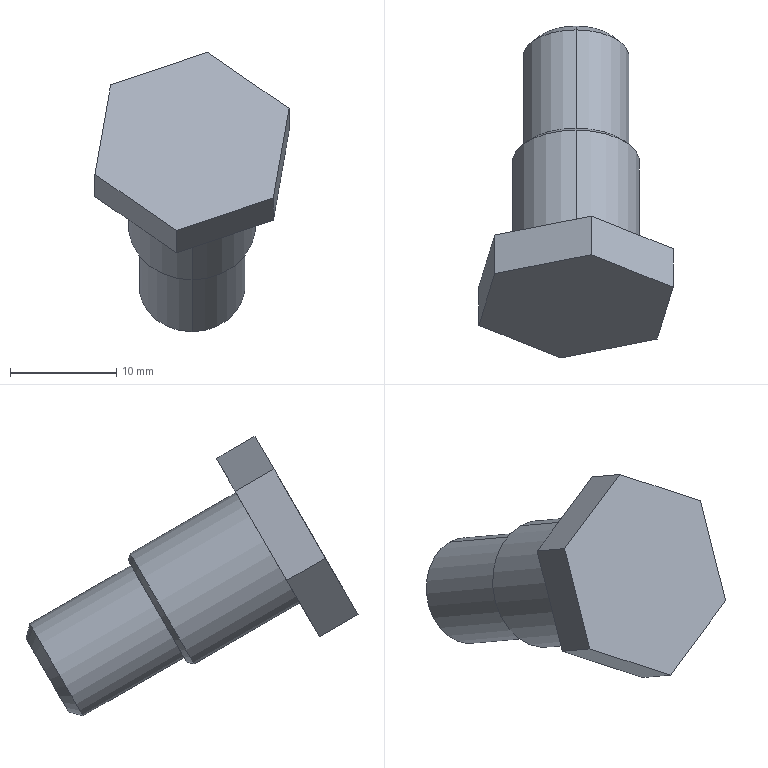Part | SolidWorks | features BaseBody 1 | 1 solid | 18 faces | box 18.291 x 31.273 x 26.332 mm | volume 3332 mm3 | plane 10 | cylinder 4 | cone 4 | commonest cylinder face diameters 10 x2 12 x2
STEP:
#1=CARTESIAN_POINT('',(-205.,-189.911,49.391));
#2=VERTEX_POINT('',#1);
#3=CARTESIAN_POINT('',(-205.,-183.911,59.783));
#4=VERTEX_POINT('',#3);
#5=CARTESIAN_POINT('',(-205.,-186.911,54.587));
#6=DIRECTION('',(0.,-0.866,0.5));
#7=DIRECTION('',(0.,-0.5,-0.866));
#8=AXIS2_PLACEMENT_3D('',#5,#6,#7);
#9=CIRCLE('',#8,6.);
#10=EDGE_CURVE('',#2,#4,#9,.T.);
#11=ORIENTED_EDGE('',*,*,#10,.T.);
#12=CARTESIAN_POINT('',(-205.,-193.871,65.533));
#13=VERTEX_POINT('',#12);
#14=CARTESIAN_POINT('',(-205.,-173.086,53.533));
#15=DIRECTION('',(0.,-0.866,0.5));
#16=VECTOR('',#15,1000.);
#17=LINE('',#14,#16);
#18=EDGE_CURVE('',#4,#13,#17,.T.);
#19=ORIENTED_EDGE('',*,*,#18,.T.);
#20=CARTESIAN_POINT('',(-205.,-199.871,55.141));
#21=VERTEX_POINT('',#20);
#22=CARTESIAN_POINT('',(-205.,-196.871,60.337));
#23=DIRECTION('',(0.,0.866,-0.5));
#24=DIRECTION('',(0.,-0.5,-0.866));
#25=AXIS2_PLACEMENT_3D('',#22,#23,#24);
#26=CIRCLE('',#25,6.);
#27=EDGE_CURVE('',#13,#21,#26,.T.);
#28=ORIENTED_EDGE('',*,*,#27,.T.);
#29=CARTESIAN_POINT('',(-205.,-179.086,43.141));
#30=DIRECTION('',(0.,-0.866,0.5));
#31=VECTOR('',#30,1000.);
#32=LINE('',#29,#31);
#33=EDGE_CURVE('',#2,#21,#32,.T.);
#34=ORIENTED_EDGE('',*,*,#33,.F.);
#35=EDGE_LOOP('',(#11,#19,#28,#34));
#36=FACE_OUTER_BOUND('',#35,.T.);
#37=CARTESIAN_POINT('',(-205.,-176.086,48.337));
#38=DIRECTION('',(0.,-0.866,0.5));
#39=DIRECTION('',(0.,-0.5,-0.866));
#40=AXIS2_PLACEMENT_3D('',#37,#38,#39);
#41=CYLINDRICAL_SURFACE('',#40,6.);
#42=ADVANCED_FACE('',(#36),#41,.T.);
#43=CARTESIAN_POINT('',(-205.,-189.228,49.574));
#44=VERTEX_POINT('',#43);
#45=CARTESIAN_POINT('',(-205.,-183.728,59.1));
#46=VERTEX_POINT('',#45);
#47=CARTESIAN_POINT('',(-205.,-186.478,54.337));
#48=DIRECTION('',(0.,-0.866,0.5));
#49=DIRECTION('',(0.,-0.5,-0.866));
#50=AXIS2_PLACEMENT_3D('',#47,#48,#49);
#51=CIRCLE('',#50,5.5);
#52=EDGE_CURVE('',#44,#46,#51,.T.);
#53=ORIENTED_EDGE('',*,*,#52,.T.);
#54=CARTESIAN_POINT('',(-205.,-183.911,59.783));
#55=DIRECTION('',(0.,-0.2588,0.9659));
#56=VECTOR('',#55,1000.);
#57=LINE('',#54,#56);
#58=EDGE_CURVE('',#46,#4,#57,.T.);
#59=ORIENTED_EDGE('',*,*,#58,.T.);
#60=ORIENTED_EDGE('',*,*,#10,.F.);
#61=CARTESIAN_POINT('',(-205.,-189.911,49.391));
#62=DIRECTION('',(0.,-0.9659,-0.2588));
#63=VECTOR('',#62,1000.);
#64=LINE('',#61,#63);
#65=EDGE_CURVE('',#44,#2,#64,.T.);
#66=ORIENTED_EDGE('',*,*,#65,.F.);
#67=EDGE_LOOP('',(#53,#59,#60,#66));
#68=FACE_OUTER_BOUND('',#67,.T.);
#69=CARTESIAN_POINT('',(-205.,-186.911,54.587));
#70=DIRECTION('',(0.,-0.866,0.5));
#71=DIRECTION('',(0.,-0.5,-0.866));
#72=AXIS2_PLACEMENT_3D('',#69,#70,#71);
#73=CONICAL_SURFACE('',#72,6.,0.7854);
#74=ADVANCED_FACE('',(#68),#73,.T.);
#75=CARTESIAN_POINT('',(-205.,-188.978,50.007));
#76=VERTEX_POINT('',#75);
#77=CARTESIAN_POINT('',(-205.,-183.978,58.667));
#78=VERTEX_POINT('',#77);
#79=CARTESIAN_POINT('',(-205.,-186.478,54.337));
#80=DIRECTION('',(0.,-0.866,0.5));
#81=DIRECTION('',(0.,0.5,0.866));
#82=AXIS2_PLACEMENT_3D('',#79,#80,#81);
#83=CIRCLE('',#82,5.);
#84=EDGE_CURVE('',#76,#78,#83,.T.);
#85=ORIENTED_EDGE('',*,*,#84,.F.);
#86=CARTESIAN_POINT('',(-205.,-179.452,44.507));
#87=VERTEX_POINT('',#86);
#88=CARTESIAN_POINT('',(-205.,-188.978,50.007));
#89=DIRECTION('',(0.,0.866,-0.5));
#90=VECTOR('',#89,1000.);
#91=LINE('',#88,#90);
#92=EDGE_CURVE('',#76,#87,#91,.T.);
#93=ORIENTED_EDGE('',*,*,#92,.T.);
#94=CARTESIAN_POINT('',(-205.,-174.452,53.167));
#95=VERTEX_POINT('',#94);
#96=CARTESIAN_POINT('',(-205.,-176.952,48.837));
#97=DIRECTION('',(0.,-0.866,0.5));
#98=DIRECTION('',(0.,0.5,0.866));
#99=AXIS2_PLACEMENT_3D('',#96,#97,#98);
#100=CIRCLE('',#99,5.);
#101=EDGE_CURVE('',#87,#95,#100,.T.);
#102=ORIENTED_EDGE('',*,*,#101,.T.);
#103=CARTESIAN_POINT('',(-205.,-183.978,58.667));
#104=DIRECTION('',(0.,0.866,-0.5));
#105=VECTOR('',#104,1000.);
#106=LINE('',#103,#105);
#107=EDGE_CURVE('',#78,#95,#106,.T.);
#108=ORIENTED_EDGE('',*,*,#107,.F.);
#109=EDGE_LOOP('',(#85,#93,#102,#108));
#110=FACE_OUTER_BOUND('',#109,.T.);
#111=CARTESIAN_POINT('',(-205.,-186.478,54.337));
#112=DIRECTION('',(0.,0.866,-0.5));
#113=DIRECTION('',(0.,0.5,0.866));
#114=AXIS2_PLACEMENT_3D('',#111,#112,#113);
#115=CYLINDRICAL_SURFACE('',#114,5.);
#116=ADVANCED_FACE('',(#110),#115,.T.);
#117=CARTESIAN_POINT('',(-205.,-178.086,44.873));
#118=VERTEX_POINT('',#117);
#119=CARTESIAN_POINT('',(-205.,-174.086,51.801));
#120=VERTEX_POINT('',#119);
#121=CARTESIAN_POINT('',(-205.,-176.086,48.337));
#122=DIRECTION('',(0.,-0.866,0.5));
#123=DIRECTION('',(0.,-0.5,-0.866));
#124=AXIS2_PLACEMENT_3D('',#121,#122,#123);
#125=CIRCLE('',#124,4.);
#126=EDGE_CURVE('',#118,#120,#125,.T.);
#127=ORIENTED_EDGE('',*,*,#126,.T.);
#128=CARTESIAN_POINT('',(-205.,-174.452,53.167));
#129=DIRECTION('',(0.,-0.2588,0.9659));
#130=VECTOR('',#129,1000.);
#131=LINE('',#128,#130);
#132=EDGE_CURVE('',#120,#95,#131,.T.);
#133=ORIENTED_EDGE('',*,*,#132,.T.);
#134=ORIENTED_EDGE('',*,*,#101,.F.);
#135=CARTESIAN_POINT('',(-205.,-179.452,44.507));
#136=DIRECTION('',(0.,-0.9659,-0.2588));
#137=VECTOR('',#136,1000.);
#138=LINE('',#135,#137);
#139=EDGE_CURVE('',#118,#87,#138,.T.);
#140=ORIENTED_EDGE('',*,*,#139,.F.);
#141=EDGE_LOOP('',(#127,#133,#134,#140));
#142=FACE_OUTER_BOUND('',#141,.T.);
#143=CARTESIAN_POINT('',(-205.,-176.952,48.837));
#144=DIRECTION('',(0.,-0.866,0.5));
#145=DIRECTION('',(0.,-0.5,-0.866));
#146=AXIS2_PLACEMENT_3D('',#143,#144,#145);
#147=CONICAL_SURFACE('',#146,5.,0.7854);
#148=ADVANCED_FACE('',(#142),#147,.T.);
#149=ORIENTED_EDGE('',*,*,#126,.F.);
#150=CARTESIAN_POINT('',(-205.,-176.086,48.337));
#151=DIRECTION('',(0.,-0.866,0.5));
#152=DIRECTION('',(0.,-0.5,-0.866));
#153=AXIS2_PLACEMENT_3D('',#150,#151,#152);
#154=CIRCLE('',#153,4.);
#155=EDGE_CURVE('',#120,#118,#154,.T.);
#156=ORIENTED_EDGE('',*,*,#155,.F.);
#157=EDGE_LOOP('',(#149,#156));
#158=FACE_OUTER_BOUND('',#157,.T.);
#159=CARTESIAN_POINT('',(-205.,-176.086,48.337));
#160=DIRECTION('',(0.,0.866,-0.5));
#161=DIRECTION('',(-1.,0.,0.));
#162=AXIS2_PLACEMENT_3D('',#159,#160,#161);
#163=PLANE('',#162);
#164=ADVANCED_FACE('',(#158),#163,.T.);
#165=CARTESIAN_POINT('',(-205.,-186.478,54.337));
#166=DIRECTION('',(0.,-0.866,0.5));
#167=DIRECTION('',(0.,0.5,0.866));
#168=AXIS2_PLACEMENT_3D('',#165,#166,#167);
#169=CIRCLE('',#168,5.);
#170=EDGE_CURVE('',#78,#76,#169,.T.);
#171=ORIENTED_EDGE('',*,*,#170,.T.);
#172=ORIENTED_EDGE('',*,*,#84,.T.);
#173=EDGE_LOOP('',(#171,#172));
#174=FACE_BOUND('',#173,.T.);
#175=ORIENTED_EDGE('',*,*,#52,.F.);
#176=CARTESIAN_POINT('',(-205.,-186.478,54.337));
#177=DIRECTION('',(0.,-0.866,0.5));
#178=DIRECTION('',(0.,-0.5,-0.866));
#179=AXIS2_PLACEMENT_3D('',#176,#177,#178);
#180=CIRCLE('',#179,5.5);
#181=EDGE_CURVE('',#46,#44,#180,.T.);
#182=ORIENTED_EDGE('',*,*,#181,.F.);
#183=EDGE_LOOP('',(#175,#182));
#184=FACE_OUTER_BOUND('',#183,.T.);
#185=CARTESIAN_POINT('',(-205.,-186.478,54.337));
#186=DIRECTION('',(0.,0.866,-0.5));
#187=DIRECTION('',(-1.,0.,0.));
#188=AXIS2_PLACEMENT_3D('',#185,#186,#187);
#189=PLANE('',#188);
#190=ADVANCED_FACE('',(#174,#184),#189,.T.);
#191=CARTESIAN_POINT('',(-205.,-196.871,60.337));
#192=DIRECTION('',(0.,0.866,-0.5));
#193=DIRECTION('',(0.,-0.5,-0.866));
#194=AXIS2_PLACEMENT_3D('',#191,#192,#193);
#195=CIRCLE('',#194,6.);
#196=EDGE_CURVE('',#21,#13,#195,.T.);
#197=ORIENTED_EDGE('',*,*,#196,.F.);
#198=ORIENTED_EDGE('',*,*,#27,.F.);
#199=EDGE_LOOP('',(#197,#198));
#200=FACE_BOUND('',#199,.T.);
#201=CARTESIAN_POINT('',(-197.342,-199.94,55.021));
#202=VERTEX_POINT('',#201);
#203=CARTESIAN_POINT('',(-206.487,-201.721,51.935));
#204=VERTEX_POINT('',#203);
#205=CARTESIAN_POINT('',(-206.487,-201.721,51.935));
#206=DIRECTION('',(-0.9318,-0.1815,-0.3144));
#207=VECTOR('',#206,1000.);
#208=LINE('',#205,#207);
#209=EDGE_CURVE('',#202,#204,#208,.T.);
#210=ORIENTED_EDGE('',*,*,#209,.T.);
#211=CARTESIAN_POINT('',(-214.145,-198.652,57.251));
#212=VERTEX_POINT('',#211);
#213=CARTESIAN_POINT('',(-206.487,-201.721,51.935));
#214=DIRECTION('',(-0.7803,0.3127,0.5416));
#215=VECTOR('',#214,1000.);
#216=LINE('',#213,#215);
#217=EDGE_CURVE('',#204,#212,#216,.T.);
#218=ORIENTED_EDGE('',*,*,#217,.T.);
#219=CARTESIAN_POINT('',(-212.658,-193.801,65.653));
#220=VERTEX_POINT('',#219);
#221=CARTESIAN_POINT('',(-214.145,-198.652,57.251));
#222=DIRECTION('',(0.1515,0.4942,0.856));
#223=VECTOR('',#222,1000.);
#224=LINE('',#221,#223);
#225=EDGE_CURVE('',#212,#220,#224,.T.);
#226=ORIENTED_EDGE('',*,*,#225,.T.);
#227=CARTESIAN_POINT('',(-203.513,-192.02,68.739));
#228=VERTEX_POINT('',#227);
#229=CARTESIAN_POINT('',(-203.513,-192.02,68.739));
#230=DIRECTION('',(0.9318,0.1815,0.3144));
#231=VECTOR('',#230,1000.);
#232=LINE('',#229,#231);
#233=EDGE_CURVE('',#220,#228,#232,.T.);
#234=ORIENTED_EDGE('',*,*,#233,.T.);
#235=CARTESIAN_POINT('',(-195.855,-195.089,63.423));
#236=VERTEX_POINT('',#235);
#237=CARTESIAN_POINT('',(-203.513,-192.02,68.739));
#238=DIRECTION('',(0.7803,-0.3127,-0.5416));
#239=VECTOR('',#238,1000.);
#240=LINE('',#237,#239);
#241=EDGE_CURVE('',#228,#236,#240,.T.);
#242=ORIENTED_EDGE('',*,*,#241,.T.);
#243=CARTESIAN_POINT('',(-195.855,-195.089,63.423));
#244=DIRECTION('',(-0.1515,-0.4942,-0.856));
#245=VECTOR('',#244,1000.);
#246=LINE('',#243,#245);
#247=EDGE_CURVE('',#236,#202,#246,.T.);
#248=ORIENTED_EDGE('',*,*,#247,.T.);
#249=EDGE_LOOP('',(#210,#218,#226,#234,#242,#248));
#250=FACE_OUTER_BOUND('',#249,.T.);
#251=CARTESIAN_POINT('',(-205.,-196.871,60.337));
#252=DIRECTION('',(0.,-0.866,0.5));
#253=DIRECTION('',(-1.,0.,0.));
#254=AXIS2_PLACEMENT_3D('',#251,#252,#253);
#255=PLANE('',#254);
#256=ADVANCED_FACE('',(#200,#250),#255,.F.);
#257=CARTESIAN_POINT('',(-195.855,-198.726,65.523));
#258=VERTEX_POINT('',#257);
#259=CARTESIAN_POINT('',(-195.855,-198.726,65.523));
#260=DIRECTION('',(0.,0.866,-0.5));
#261=VECTOR('',#260,1000.);
#262=LINE('',#259,#261);
#263=EDGE_CURVE('',#258,#236,#262,.T.);
#264=ORIENTED_EDGE('',*,*,#263,.T.);
#265=ORIENTED_EDGE('',*,*,#241,.F.);
#266=CARTESIAN_POINT('',(-203.513,-195.657,70.839));
#267=VERTEX_POINT('',#266);
#268=CARTESIAN_POINT('',(-203.513,-195.657,70.839));
#269=DIRECTION('',(0.,-0.866,0.5));
#270=VECTOR('',#269,1000.);
#271=LINE('',#268,#270);
#272=EDGE_CURVE('',#228,#267,#271,.T.);
#273=ORIENTED_EDGE('',*,*,#272,.T.);
#274=CARTESIAN_POINT('',(-195.855,-198.726,65.523));
#275=DIRECTION('',(-0.7803,0.3127,0.5416));
#276=VECTOR('',#275,1000.);
#277=LINE('',#274,#276);
#278=EDGE_CURVE('',#258,#267,#277,.T.);
#279=ORIENTED_EDGE('',*,*,#278,.F.);
#280=EDGE_LOOP('',(#264,#265,#273,#279));
#281=FACE_OUTER_BOUND('',#280,.T.);
#282=CARTESIAN_POINT('',(-195.855,-198.726,65.523));
#283=DIRECTION('',(-0.6254,-0.3901,-0.6757));
#284=DIRECTION('',(-0.7339,0.,0.6793));
#285=AXIS2_PLACEMENT_3D('',#282,#283,#284);
#286=PLANE('',#285);
#287=ADVANCED_FACE('',(#281),#286,.F.);
#288=ORIENTED_EDGE('',*,*,#272,.F.);
#289=ORIENTED_EDGE('',*,*,#233,.F.);
#290=CARTESIAN_POINT('',(-212.658,-197.439,67.753));
#291=VERTEX_POINT('',#290);
#292=CARTESIAN_POINT('',(-212.658,-193.801,65.653));
#293=DIRECTION('',(0.,-0.866,0.5));
#294=VECTOR('',#293,1000.);
#295=LINE('',#292,#294);
#296=EDGE_CURVE('',#220,#291,#295,.T.);
#297=ORIENTED_EDGE('',*,*,#296,.T.);
#298=CARTESIAN_POINT('',(-203.513,-195.657,70.839));
#299=DIRECTION('',(-0.9318,-0.1815,-0.3144));
#300=VECTOR('',#299,1000.);
#301=LINE('',#298,#300);
#302=EDGE_CURVE('',#267,#291,#301,.T.);
#303=ORIENTED_EDGE('',*,*,#302,.F.);
#304=EDGE_LOOP('',(#288,#289,#297,#303));
#305=FACE_OUTER_BOUND('',#304,.T.);
#306=CARTESIAN_POINT('',(-203.513,-195.657,70.839));
#307=DIRECTION('',(0.363,-0.4659,-0.8069));
#308=DIRECTION('',(0.,-0.866,0.5));
#309=AXIS2_PLACEMENT_3D('',#306,#307,#308);
#310=PLANE('',#309);
#311=ADVANCED_FACE('',(#305),#310,.F.);
#312=ORIENTED_EDGE('',*,*,#296,.F.);
#313=ORIENTED_EDGE('',*,*,#225,.F.);
#314=CARTESIAN_POINT('',(-214.145,-202.29,59.351));
#315=VERTEX_POINT('',#314);
#316=CARTESIAN_POINT('',(-214.145,-198.652,57.251));
#317=DIRECTION('',(0.,-0.866,0.5));
#318=VECTOR('',#317,1000.);
#319=LINE('',#316,#318);
#320=EDGE_CURVE('',#212,#315,#319,.T.);
#321=ORIENTED_EDGE('',*,*,#320,.T.);
#322=CARTESIAN_POINT('',(-212.658,-197.439,67.753));
#323=DIRECTION('',(-0.1515,-0.4942,-0.856));
#324=VECTOR('',#323,1000.);
#325=LINE('',#322,#324);
#326=EDGE_CURVE('',#291,#315,#325,.T.);
#327=ORIENTED_EDGE('',*,*,#326,.F.);
#328=EDGE_LOOP('',(#312,#313,#321,#327));
#329=FACE_OUTER_BOUND('',#328,.T.);
#330=CARTESIAN_POINT('',(-212.658,-197.439,67.753));
#331=DIRECTION('',(0.9885,-0.07575,-0.1312));
#332=DIRECTION('',(0.,-0.866,0.5));
#333=AXIS2_PLACEMENT_3D('',#330,#331,#332);
#334=PLANE('',#333);
#335=ADVANCED_FACE('',(#329),#334,.F.);
#336=ORIENTED_EDGE('',*,*,#320,.F.);
#337=ORIENTED_EDGE('',*,*,#217,.F.);
#338=CARTESIAN_POINT('',(-206.487,-205.359,54.035));
#339=VERTEX_POINT('',#338);
#340=CARTESIAN_POINT('',(-206.487,-205.359,54.035));
#341=DIRECTION('',(0.,-0.866,0.5));
#342=VECTOR('',#341,1000.);
#343=LINE('',#340,#342);
#344=EDGE_CURVE('',#204,#339,#343,.T.);
#345=ORIENTED_EDGE('',*,*,#344,.T.);
#346=CARTESIAN_POINT('',(-214.145,-202.29,59.351));
#347=DIRECTION('',(0.7803,-0.3127,-0.5416));
#348=VECTOR('',#347,1000.);
#349=LINE('',#346,#348);
#350=EDGE_CURVE('',#315,#339,#349,.T.);
#351=ORIENTED_EDGE('',*,*,#350,.F.);
#352=EDGE_LOOP('',(#336,#337,#345,#351));
#353=FACE_OUTER_BOUND('',#352,.T.);
#354=CARTESIAN_POINT('',(-214.145,-202.29,59.351));
#355=DIRECTION('',(0.6254,0.3901,0.6757));
#356=DIRECTION('',(0.5293,-0.8485,0.));
#357=AXIS2_PLACEMENT_3D('',#354,#355,#356);
#358=PLANE('',#357);
#359=ADVANCED_FACE('',(#353),#358,.F.);
#360=ORIENTED_EDGE('',*,*,#344,.F.);
#361=ORIENTED_EDGE('',*,*,#209,.F.);
#362=CARTESIAN_POINT('',(-197.342,-203.577,57.121));
#363=VERTEX_POINT('',#362);
#364=CARTESIAN_POINT('',(-197.342,-199.94,55.021));
#365=DIRECTION('',(0.,-0.866,0.5));
#366=VECTOR('',#365,1000.);
#367=LINE('',#364,#366);
#368=EDGE_CURVE('',#202,#363,#367,.T.);
#369=ORIENTED_EDGE('',*,*,#368,.T.);
#370=CARTESIAN_POINT('',(-206.487,-205.359,54.035));
#371=DIRECTION('',(0.9318,0.1815,0.3144));
#372=VECTOR('',#371,1000.);
#373=LINE('',#370,#372);
#374=EDGE_CURVE('',#339,#363,#373,.T.);
#375=ORIENTED_EDGE('',*,*,#374,.F.);
#376=EDGE_LOOP('',(#360,#361,#369,#375));
#377=FACE_OUTER_BOUND('',#376,.T.);
#378=CARTESIAN_POINT('',(-206.487,-205.359,54.035));
#379=DIRECTION('',(-0.363,0.4659,0.8069));
#380=DIRECTION('',(0.7888,0.6146,0.));
#381=AXIS2_PLACEMENT_3D('',#378,#379,#380);
#382=PLANE('',#381);
#383=ADVANCED_FACE('',(#377),#382,.F.);
#384=ORIENTED_EDGE('',*,*,#368,.F.);
#385=ORIENTED_EDGE('',*,*,#247,.F.);
#386=ORIENTED_EDGE('',*,*,#263,.F.);
#387=CARTESIAN_POINT('',(-197.342,-203.577,57.121));
#388=DIRECTION('',(0.1515,0.4942,0.856));
#389=VECTOR('',#388,1000.);
#390=LINE('',#387,#389);
#391=EDGE_CURVE('',#363,#258,#390,.T.);
#392=ORIENTED_EDGE('',*,*,#391,.F.);
#393=EDGE_LOOP('',(#384,#385,#386,#392));
#394=FACE_OUTER_BOUND('',#393,.T.);
#395=CARTESIAN_POINT('',(-197.342,-203.577,57.121));
#396=DIRECTION('',(-0.9885,0.07575,0.1312));
#397=DIRECTION('',(0.07641,0.9971,0.));
#398=AXIS2_PLACEMENT_3D('',#395,#396,#397);
#399=PLANE('',#398);
#400=ADVANCED_FACE('',(#394),#399,.F.);
#401=ORIENTED_EDGE('',*,*,#374,.T.);
#402=ORIENTED_EDGE('',*,*,#391,.T.);
#403=ORIENTED_EDGE('',*,*,#278,.T.);
#404=ORIENTED_EDGE('',*,*,#302,.T.);
#405=ORIENTED_EDGE('',*,*,#326,.T.);
#406=ORIENTED_EDGE('',*,*,#350,.T.);
#407=EDGE_LOOP('',(#401,#402,#403,#404,#405,#406));
#408=FACE_OUTER_BOUND('',#407,.T.);
#409=CARTESIAN_POINT('',(-205.,-200.508,62.437));
#410=DIRECTION('',(0.,-0.866,0.5));
#411=DIRECTION('',(-1.,0.,0.));
#412=AXIS2_PLACEMENT_3D('',#409,#410,#411);
#413=PLANE('',#412);
#414=ADVANCED_FACE('',(#408),#413,.T.);
#415=ORIENTED_EDGE('',*,*,#132,.F.);
#416=ORIENTED_EDGE('',*,*,#155,.T.);
#417=ORIENTED_EDGE('',*,*,#139,.T.);
#418=CARTESIAN_POINT('',(-205.,-176.952,48.837));
#419=DIRECTION('',(0.,-0.866,0.5));
#420=DIRECTION('',(0.,0.5,0.866));
#421=AXIS2_PLACEMENT_3D('',#418,#419,#420);
#422=CIRCLE('',#421,5.);
#423=EDGE_CURVE('',#95,#87,#422,.T.);
#424=ORIENTED_EDGE('',*,*,#423,.F.);
#425=EDGE_LOOP('',(#415,#416,#417,#424));
#426=FACE_OUTER_BOUND('',#425,.T.);
#427=CARTESIAN_POINT('',(-205.,-176.952,48.837));
#428=DIRECTION('',(0.,-0.866,0.5));
#429=DIRECTION('',(0.,-0.5,-0.866));
#430=AXIS2_PLACEMENT_3D('',#427,#428,#429);
#431=CONICAL_SURFACE('',#430,5.,0.7854);
#432=ADVANCED_FACE('',(#426),#431,.T.);
#433=ORIENTED_EDGE('',*,*,#92,.F.);
#434=ORIENTED_EDGE('',*,*,#170,.F.);
#435=ORIENTED_EDGE('',*,*,#107,.T.);
#436=ORIENTED_EDGE('',*,*,#423,.T.);
#437=EDGE_LOOP('',(#433,#434,#435,#436));
#438=FACE_OUTER_BOUND('',#437,.T.);
#439=CARTESIAN_POINT('',(-205.,-186.478,54.337));
#440=DIRECTION('',(0.,0.866,-0.5));
#441=DIRECTION('',(0.,0.5,0.866));
#442=AXIS2_PLACEMENT_3D('',#439,#440,#441);
#443=CYLINDRICAL_SURFACE('',#442,5.);
#444=ADVANCED_FACE('',(#438),#443,.T.);
#445=ORIENTED_EDGE('',*,*,#58,.F.);
#446=ORIENTED_EDGE('',*,*,#181,.T.);
#447=ORIENTED_EDGE('',*,*,#65,.T.);
#448=CARTESIAN_POINT('',(-205.,-186.911,54.587));
#449=DIRECTION('',(0.,-0.866,0.5));
#450=DIRECTION('',(0.,-0.5,-0.866));
#451=AXIS2_PLACEMENT_3D('',#448,#449,#450);
#452=CIRCLE('',#451,6.);
#453=EDGE_CURVE('',#4,#2,#452,.T.);
#454=ORIENTED_EDGE('',*,*,#453,.F.);
#455=EDGE_LOOP('',(#445,#446,#447,#454));
#456=FACE_OUTER_BOUND('',#455,.T.);
#457=CARTESIAN_POINT('',(-205.,-186.911,54.587));
#458=DIRECTION('',(0.,-0.866,0.5));
#459=DIRECTION('',(0.,-0.5,-0.866));
#460=AXIS2_PLACEMENT_3D('',#457,#458,#459);
#461=CONICAL_SURFACE('',#460,6.,0.7854);
#462=ADVANCED_FACE('',(#456),#461,.T.);
#463=ORIENTED_EDGE('',*,*,#18,.F.);
#464=ORIENTED_EDGE('',*,*,#453,.T.);
#465=ORIENTED_EDGE('',*,*,#33,.T.);
#466=ORIENTED_EDGE('',*,*,#196,.T.);
#467=EDGE_LOOP('',(#463,#464,#465,#466));
#468=FACE_OUTER_BOUND('',#467,.T.);
#469=CARTESIAN_POINT('',(-205.,-176.086,48.337));
#470=DIRECTION('',(0.,-0.866,0.5));
#471=DIRECTION('',(0.,-0.5,-0.866));
#472=AXIS2_PLACEMENT_3D('',#469,#470,#471);
#473=CYLINDRICAL_SURFACE('',#472,6.);
#474=ADVANCED_FACE('',(#468),#473,.T.);
#475=CLOSED_SHELL('',(#42,#74,#116,#148,#164,#190,#256,#287,#311,#335,#359,#383,#400,#414,#432,#444,#462,#474));
#476=MANIFOLD_SOLID_BREP('',#475);
#477=CARTESIAN_POINT('',(0.,0.,0.));
#478=DIRECTION('',(0.,0.,1.));
#479=DIRECTION('',(1.,0.,0.));
#480=AXIS2_PLACEMENT_3D('',#477,#478,#479);
#481=(LENGTH_UNIT()NAMED_UNIT(*)SI_UNIT(.MILLI.,.METRE.));
#482=UNCERTAINTY_MEASURE_WITH_UNIT(LENGTH_MEASURE(0.00001),#481,'','');
#483=(NAMED_UNIT(*)PLANE_ANGLE_UNIT()SI_UNIT($,.RADIAN.));
#484=(NAMED_UNIT(*)SI_UNIT($,.STERADIAN.)SOLID_ANGLE_UNIT());
#485=(GEOMETRIC_REPRESENTATION_CONTEXT(3)GLOBAL_UNCERTAINTY_ASSIGNED_CONTEXT((#482))GLOBAL_UNIT_ASSIGNED_CONTEXT((#481,#483,#484))REPRESENTATION_CONTEXT('',''));
#486=ADVANCED_BREP_SHAPE_REPRESENTATION('',(#476,#480),#485);